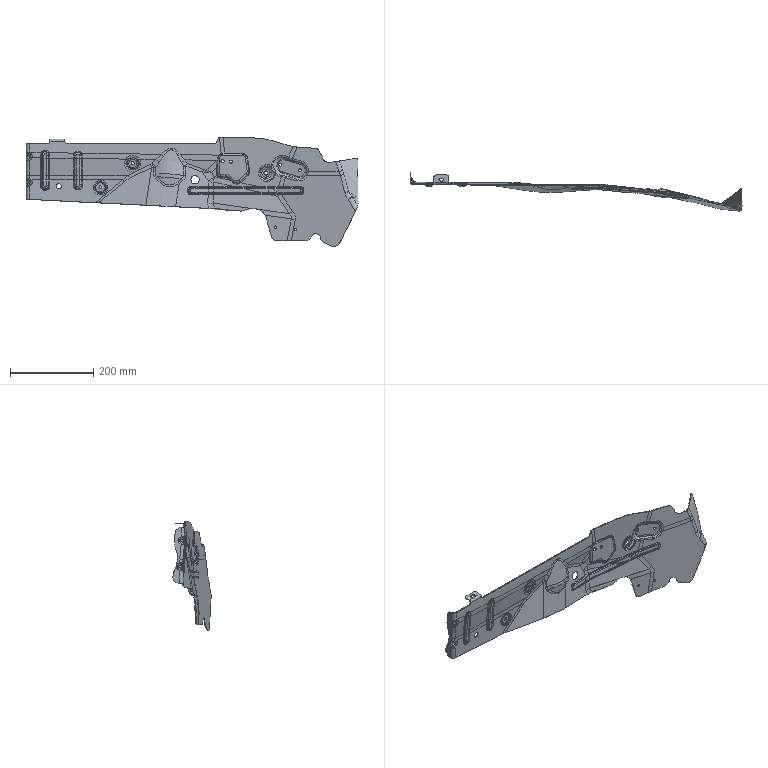Part | 1 solid | 930 faces | box 798.571 x 92.352 x 263.155 mm | volume 208274 mm3 | spline 715 | cylinder 147 | plane 56 | other 6 | sphere 6 | commonest cylinder face diameters 10 x27 13 x16 7 x15 200 x11 157 x6 160 x6